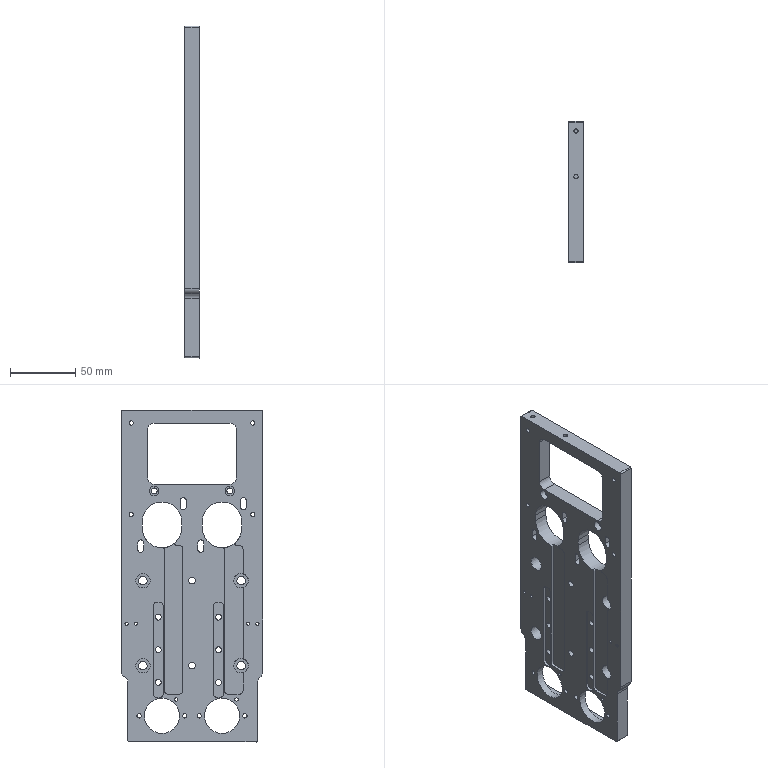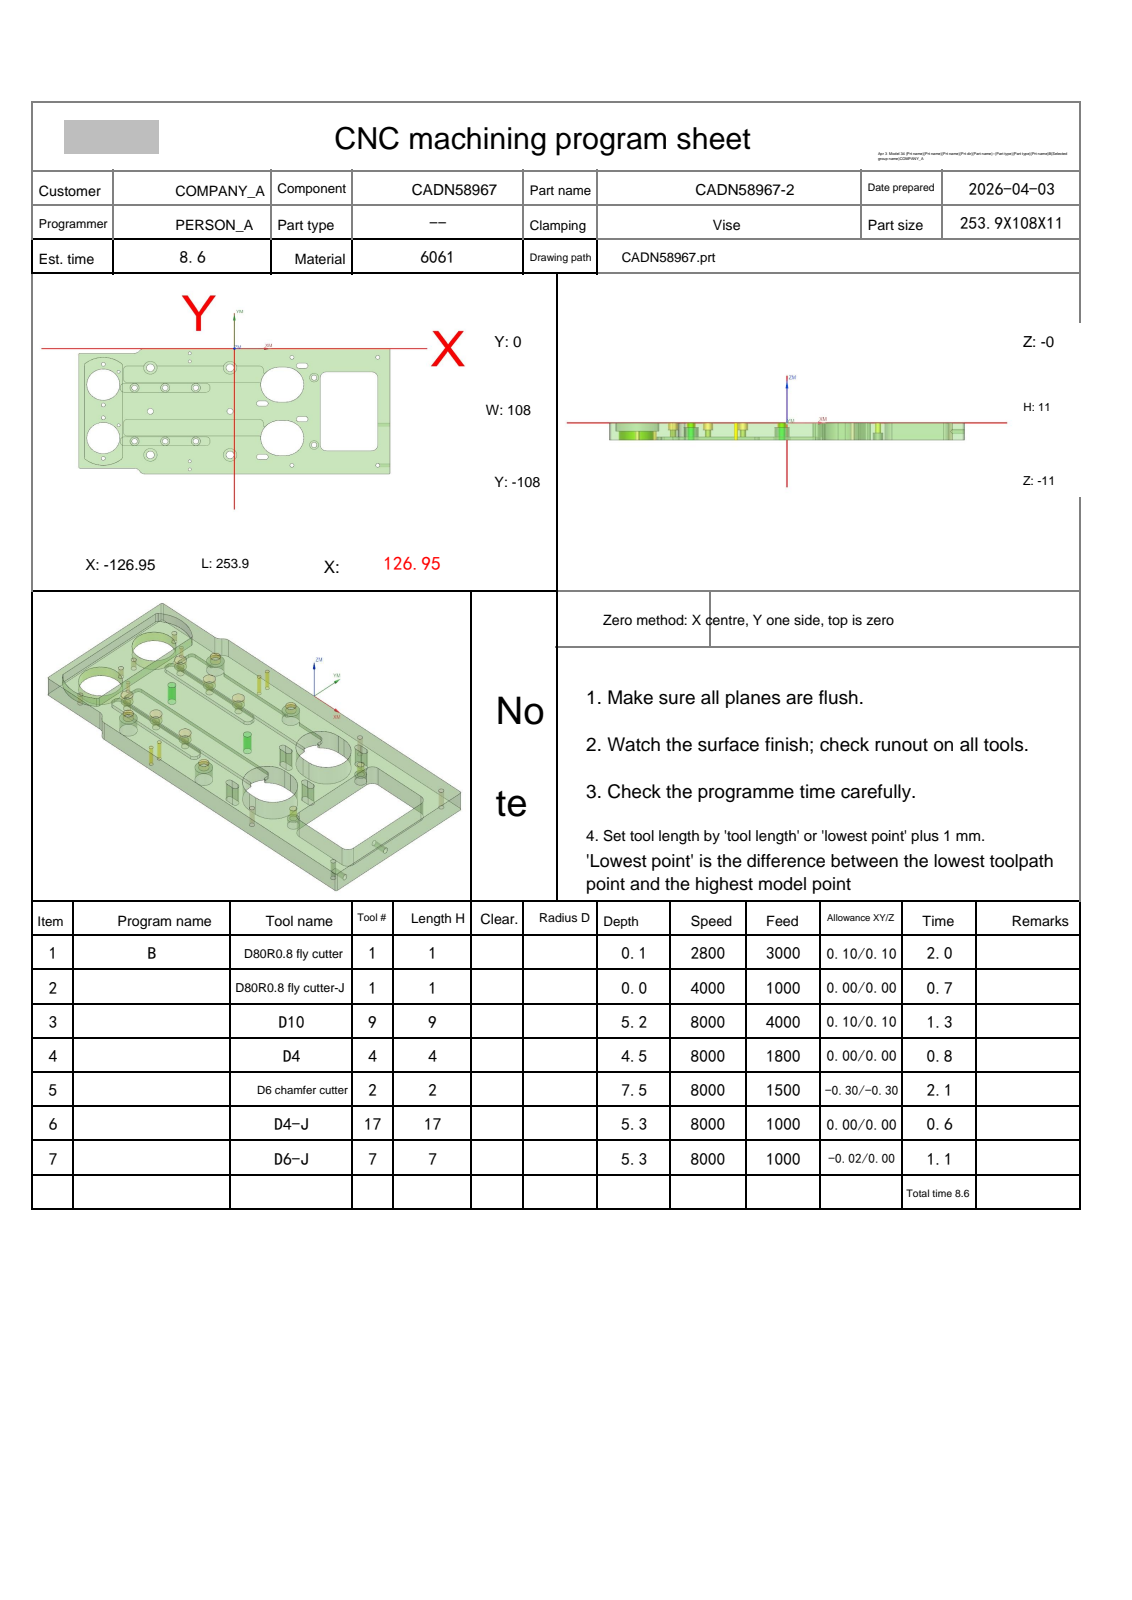NC program | NX | posted by the shop | part box 11 x 108 x 253.9 mm
Lines 1 to 1505 of 3878:
%
O0001
(Machine time: 9.94 MIN)
(===Total Tool:6===)
(T1=D80R0.8 fly cutter D=80.  R=0.8  D-  H01 Z=-0.   )
(T9=D10     D=10.  R=0.   D-  H09 Z=-5.2  )
(T4=D4      D=4.   R=0.   D-  H04 Z=-4.5  )
(T2=D6 chamfer cutter   D=6.   R=0.   D-  H02 Z=-7.5  )
(T17=D4-J   D=4.   R=0.   D-  H17 Z=-5.3  )
(T7=D6-J    D=6.   R=0.   D7  H07 Z=-5.3  )
G80 G90 G17 G49 G40
G91 G28 Z0
M01
N1 T01 M06
(D80R0.8 fly cutter  D=80. R=0.8 H=01 ce=0.10 di=0.10)
G00 G90 G54 X179.047 Y-84.097 M03 S2800
G43 H01 Z20.
M08
Z5.513
G01 Z3.513 F3000.
X167.047
X-159.05
G02 X-167.047 Y-76.101 I.003 J8.
G01 Y-39.263
G02 X-159.047 Y-31.263 I8. J0.0
G01 X167.047
X179.047
Z5.513
G00 Y-84.097
Z5.025
G01 Z3.025
X167.047
X-159.05
G02 X-167.047 Y-76.101 I.003 J8.
G01 Y-39.263
G02 X-159.047 Y-31.263 I8. J0.0
G01 X167.047
X179.047
Z5.025
G00 Y-84.097
Z4.538
G01 Z2.538
X167.047
X-159.05
G02 X-167.047 Y-76.101 I.003 J8.
G01 Y-39.263
G02 X-159.047 Y-31.263 I8. J0.0
G01 X167.047
X179.047
Z4.538
G00 Y-84.097
Z4.05
G01 Z2.05
X167.047
X-159.05
G02 X-167.047 Y-76.101 I.003 J8.
G01 Y-39.263
G02 X-159.047 Y-31.263 I8. J0.0
G01 X167.047
X179.047
Z4.05
G00 Y-84.097
Z3.563
G01 Z1.563
X167.047
X-159.05
G02 X-167.047 Y-76.101 I.003 J8.
G01 Y-39.263
G02 X-159.047 Y-31.263 I8. J0.0
G01 X167.047
X179.047
Z3.563
G00 Y-84.097
Z3.075
G01 Z1.075
X167.047
X-159.05
G02 X-167.047 Y-76.101 I.003 J8.
G01 Y-39.263
G02 X-159.047 Y-31.263 I8. J0.0
G01 X167.047
X179.047
Z3.075
G00 Y-84.097
Z2.588
G01 Z.588
X167.047
X-159.05
G02 X-167.047 Y-76.101 I.003 J8.
G01 Y-39.263
G02 X-159.047 Y-31.263 I8. J0.0
G01 X167.047
X179.047
Z2.588
G00 Y-84.097
Z2.1
G01 Z.1
X167.047
X-159.05
G02 X-167.047 Y-76.101 I.003 J8.
G01 Y-39.263
G02 X-159.047 Y-31.263 I8. J0.0
G01 X167.047
X179.047
Z2.1
G00 Z20.
G91 G28 Z0.0
M05
M09
G91 G28 Z0.0
M01
N2 T01 M06
(D80R0.8 fly cutter-J  D=80. R=0.8 H=01 ce=0.00 di=0.00)
G00 G90 G54 X178.949 Y-83.999 M03 S4000
G43 H01 Z20.
M08
Z2.
G01 Z0.0 F1000.
X166.949
X-158.953
G02 X-166.949 Y-76.003 I.004 J8.
G01 Y-39.361
G02 X-158.949 Y-31.361 I8. J0.0
G01 X166.949
X178.949
Z2.
G00 Z20.
G91 G28 Z0.0
M05
M09
G91 G28 Z0.0
M01
N3 T09 M06
(D10  D=10. R=0. H=09 ce=0.10 di=0.10)
G00 G90 G54 X-104.445 Y-49.592 M03 S8000
G43 H09 Z13.814
M08
Z1.5
G03 X-104.445 Y-49.592 Z.018 I-.905 J-4.408 F4000.
X-109.85 Y-54. Z-.4 I-.905 J-4.408
G01 Y-86.718
G03 X-109.044 Y-87.697 I1. J.002
X-106.95 Y-87.9 I2.094 J10.697
X-104.856 Y-87.697 I0.0 J10.9
X-104.05 Y-86.718 I-.194 J.981
G01 Y-21.282
G03 X-104.856 Y-20.303 I-1. J-.002
X-106.95 Y-20.1 I-2.094 J-10.697
X-109.044 Y-20.303 I0.0 J-10.9
X-109.85 Y-21.282 I.194 J-.981
G01 Y-50.965
G02 X-110.295 Y-51.797 I-1. J0.0
G01 X-116.905 Y-56.203
G03 X-117.35 Y-57.035 I.555 J-.832
G01 Y-92.179
G03 X-106.95 Y-95.4 I10.4 J15.179
X-96.55 Y-92.179 I0.0 J18.4
G01 Y-15.821
G03 X-106.95 Y-12.6 I-10.4 J-15.179
X-117.35 Y-15.821 I0.0 J-18.4
G01 Y-59.
Y-59.5
X-114.35
Z1.1
G00 X-104.445 Y-49.592
G03 X-104.445 Y-49.592 Z-.382 I-.905 J-4.408
X-109.85 Y-54. Z-.8 I-.905 J-4.408
G01 Y-86.718
G03 X-109.044 Y-87.697 I1. J.002
X-106.95 Y-87.9 I2.094 J10.697
X-104.856 Y-87.697 I0.0 J10.9
X-104.05 Y-86.718 I-.194 J.981
G01 Y-21.282
G03 X-104.856 Y-20.303 I-1. J-.002
X-106.95 Y-20.1 I-2.094 J-10.697
X-109.044 Y-20.303 I0.0 J-10.9
X-109.85 Y-21.282 I.194 J-.981
G01 Y-50.965
G02 X-110.295 Y-51.797 I-1. J0.0
G01 X-116.905 Y-56.203
G03 X-117.35 Y-57.035 I.555 J-.832
G01 Y-92.179
G03 X-106.95 Y-95.4 I10.4 J15.179
X-96.55 Y-92.179 I0.0 J18.4
G01 Y-15.821
G03 X-106.95 Y-12.6 I-10.4 J-15.179
X-117.35 Y-15.821 I0.0 J-18.4
G01 Y-59.
Y-59.5
X-114.35
Z.7
G00 X-104.445 Y-49.592
G03 X-104.445 Y-49.592 Z-.782 I-.905 J-4.408
X-109.85 Y-54. Z-1.2 I-.905 J-4.408
G01 Y-86.718
G03 X-109.044 Y-87.697 I1. J.002
X-106.95 Y-87.9 I2.094 J10.697
X-104.856 Y-87.697 I0.0 J10.9
X-104.05 Y-86.718 I-.194 J.981
G01 Y-21.282
G03 X-104.856 Y-20.303 I-1. J-.002
X-106.95 Y-20.1 I-2.094 J-10.697
X-109.044 Y-20.303 I0.0 J-10.9
X-109.85 Y-21.282 I.194 J-.981
G01 Y-50.965
G02 X-110.295 Y-51.797 I-1. J0.0
G01 X-116.905 Y-56.203
G03 X-117.35 Y-57.035 I.555 J-.832
G01 Y-92.179
G03 X-106.95 Y-95.4 I10.4 J15.179
X-96.55 Y-92.179 I0.0 J18.4
G01 Y-15.821
G03 X-106.95 Y-12.6 I-10.4 J-15.179
X-117.35 Y-15.821 I0.0 J-18.4
G01 Y-59.
Y-59.5
X-114.35
Z.3
G00 X-104.445 Y-49.592
G03 X-104.445 Y-49.592 Z-1.182 I-.905 J-4.408
X-109.85 Y-54. Z-1.6 I-.905 J-4.408
G01 Y-86.718
G03 X-109.044 Y-87.697 I1. J.002
X-106.95 Y-87.9 I2.094 J10.697
X-104.856 Y-87.697 I0.0 J10.9
X-104.05 Y-86.718 I-.194 J.981
G01 Y-21.282
G03 X-104.856 Y-20.303 I-1. J-.002
X-106.95 Y-20.1 I-2.094 J-10.697
X-109.044 Y-20.303 I0.0 J-10.9
X-109.85 Y-21.282 I.194 J-.981
G01 Y-50.965
G02 X-110.295 Y-51.797 I-1. J0.0
G01 X-116.905 Y-56.203
G03 X-117.35 Y-57.035 I.555 J-.832
G01 Y-92.179
G03 X-106.95 Y-95.4 I10.4 J15.179
X-96.55 Y-92.179 I0.0 J18.4
G01 Y-15.821
G03 X-106.95 Y-12.6 I-10.4 J-15.179
X-117.35 Y-15.821 I0.0 J-18.4
G01 Y-59.
Y-59.5
X-114.35
Z-.1
G00 X-104.445 Y-49.592
G03 X-104.445 Y-49.592 Z-1.582 I-.905 J-4.408
X-109.85 Y-54. Z-2. I-.905 J-4.408
G01 Y-86.718
G03 X-109.044 Y-87.697 I1. J.002
X-106.95 Y-87.9 I2.094 J10.697
X-104.856 Y-87.697 I0.0 J10.9
X-104.05 Y-86.718 I-.194 J.981
G01 Y-21.282
G03 X-104.856 Y-20.303 I-1. J-.002
X-106.95 Y-20.1 I-2.094 J-10.697
X-109.044 Y-20.303 I0.0 J-10.9
X-109.85 Y-21.282 I.194 J-.981
G01 Y-50.965
G02 X-110.295 Y-51.797 I-1. J0.0
G01 X-116.905 Y-56.203
G03 X-117.35 Y-57.035 I.555 J-.832
G01 Y-92.179
G03 X-106.95 Y-95.4 I10.4 J15.179
X-96.55 Y-92.179 I0.0 J18.4
G01 Y-15.821
G03 X-106.95 Y-12.6 I-10.4 J-15.179
X-117.35 Y-15.821 I0.0 J-18.4
G01 Y-59.
Y-59.5
X-114.35
Z-.5
G00 X-104.445 Y-49.592
G03 X-104.445 Y-49.592 Z-1.982 I-.905 J-4.408
X-109.85 Y-54. Z-2.4 I-.905 J-4.408
G01 Y-86.718
G03 X-109.044 Y-87.697 I1. J.002
X-106.95 Y-87.9 I2.094 J10.697
X-104.856 Y-87.697 I0.0 J10.9
X-104.05 Y-86.718 I-.194 J.981
G01 Y-21.282
G03 X-104.856 Y-20.303 I-1. J-.002
X-106.95 Y-20.1 I-2.094 J-10.697
X-109.044 Y-20.303 I0.0 J-10.9
X-109.85 Y-21.282 I.194 J-.981
G01 Y-50.965
G02 X-110.295 Y-51.797 I-1. J0.0
G01 X-116.905 Y-56.203
G03 X-117.35 Y-57.035 I.555 J-.832
G01 Y-92.179
G03 X-106.95 Y-95.4 I10.4 J15.179
X-96.55 Y-92.179 I0.0 J18.4
G01 Y-15.821
G03 X-106.95 Y-12.6 I-10.4 J-15.179
X-117.35 Y-15.821 I0.0 J-18.4
G01 Y-59.
Y-59.5
X-114.35
Z-.9
G00 X-104.445 Y-49.592
G03 X-104.445 Y-49.592 Z-2.382 I-.905 J-4.408
X-109.85 Y-54. Z-2.8 I-.905 J-4.408
G01 Y-86.718
G03 X-109.044 Y-87.697 I1. J.002
X-106.95 Y-87.9 I2.094 J10.697
X-104.856 Y-87.697 I0.0 J10.9
X-104.05 Y-86.718 I-.194 J.981
G01 Y-21.282
G03 X-104.856 Y-20.303 I-1. J-.002
X-106.95 Y-20.1 I-2.094 J-10.697
X-109.044 Y-20.303 I0.0 J-10.9
X-109.85 Y-21.282 I.194 J-.981
G01 Y-50.965
G02 X-110.295 Y-51.797 I-1. J0.0
G01 X-116.905 Y-56.203
G03 X-117.35 Y-57.035 I.555 J-.832
G01 Y-92.179
G03 X-106.95 Y-95.4 I10.4 J15.179
X-96.55 Y-92.179 I0.0 J18.4
G01 Y-15.821
G03 X-106.95 Y-12.6 I-10.4 J-15.179
X-117.35 Y-15.821 I0.0 J-18.4
G01 Y-59.
Y-59.5
X-114.35
Z-1.3
G00 X-104.445 Y-49.592
G03 X-104.445 Y-49.592 Z-2.782 I-.905 J-4.408
X-109.85 Y-54. Z-3.2 I-.905 J-4.408
G01 Y-86.718
G03 X-109.044 Y-87.697 I1. J.002
X-106.95 Y-87.9 I2.094 J10.697
X-104.856 Y-87.697 I0.0 J10.9
X-104.05 Y-86.718 I-.194 J.981
G01 Y-21.282
G03 X-104.856 Y-20.303 I-1. J-.002
X-106.95 Y-20.1 I-2.094 J-10.697
X-109.044 Y-20.303 I0.0 J-10.9
X-109.85 Y-21.282 I.194 J-.981
G01 Y-50.965
G02 X-110.295 Y-51.797 I-1. J0.0
G01 X-116.905 Y-56.203
G03 X-117.35 Y-57.035 I.555 J-.832
G01 Y-92.179
G03 X-106.95 Y-95.4 I10.4 J15.179
X-96.55 Y-92.179 I0.0 J18.4
G01 Y-15.821
G03 X-106.95 Y-12.6 I-10.4 J-15.179
X-117.35 Y-15.821 I0.0 J-18.4
G01 Y-59.
Y-59.5
X-114.35
Z-1.7
G00 X-104.445 Y-49.592
G03 X-104.445 Y-49.592 Z-3.182 I-.905 J-4.408
X-109.85 Y-54. Z-3.6 I-.905 J-4.408
G01 Y-86.718
G03 X-109.044 Y-87.697 I1. J.002
X-106.95 Y-87.9 I2.094 J10.697
X-104.856 Y-87.697 I0.0 J10.9
X-104.05 Y-86.718 I-.194 J.981
G01 Y-21.282
G03 X-104.856 Y-20.303 I-1. J-.002
X-106.95 Y-20.1 I-2.094 J-10.697
X-109.044 Y-20.303 I0.0 J-10.9
X-109.85 Y-21.282 I.194 J-.981
G01 Y-50.965
G02 X-110.295 Y-51.797 I-1. J0.0
G01 X-116.905 Y-56.203
G03 X-117.35 Y-57.035 I.555 J-.832
G01 Y-92.179
G03 X-106.95 Y-95.4 I10.4 J15.179
X-96.55 Y-92.179 I0.0 J18.4
G01 Y-15.821
G03 X-106.95 Y-12.6 I-10.4 J-15.179
X-117.35 Y-15.821 I0.0 J-18.4
G01 Y-59.
Y-59.5
X-114.35
Z-2.1
G00 X-104.445 Y-49.592
G03 X-104.445 Y-49.592 Z-3.582 I-.905 J-4.408
X-109.85 Y-54. Z-4. I-.905 J-4.408
G01 Y-86.718
G03 X-109.044 Y-87.697 I1. J.002
X-106.95 Y-87.9 I2.094 J10.697
X-104.856 Y-87.697 I0.0 J10.9
X-104.05 Y-86.718 I-.194 J.981
G01 Y-21.282
G03 X-104.856 Y-20.303 I-1. J-.002
X-106.95 Y-20.1 I-2.094 J-10.697
X-109.044 Y-20.303 I0.0 J-10.9
X-109.85 Y-21.282 I.194 J-.981
G01 Y-50.965
G02 X-110.295 Y-51.797 I-1. J0.0
G01 X-116.905 Y-56.203
G03 X-117.35 Y-57.035 I.555 J-.832
G01 Y-92.179
G03 X-106.95 Y-95.4 I10.4 J15.179
X-96.55 Y-92.179 I0.0 J18.4
G01 Y-15.821
G03 X-106.95 Y-12.6 I-10.4 J-15.179
X-117.35 Y-15.821 I0.0 J-18.4
G01 Y-59.
Y-59.5
X-114.35
Z-2.5
G00 X-104.445 Y-49.592
G03 X-104.445 Y-49.592 Z-3.982 I-.905 J-4.408
X-109.85 Y-54. Z-4.4 I-.905 J-4.408
G01 Y-86.718
G03 X-109.044 Y-87.697 I1. J.002
X-106.95 Y-87.9 I2.094 J10.697
X-104.856 Y-87.697 I0.0 J10.9
X-104.05 Y-86.718 I-.194 J.981
G01 Y-21.282
G03 X-104.856 Y-20.303 I-1. J-.002
X-106.95 Y-20.1 I-2.094 J-10.697
X-109.044 Y-20.303 I0.0 J-10.9
X-109.85 Y-21.282 I.194 J-.981
G01 Y-50.965
G02 X-110.295 Y-51.797 I-1. J0.0
G01 X-116.905 Y-56.203
G03 X-117.35 Y-57.035 I.555 J-.832
G01 Y-92.179
G03 X-106.95 Y-95.4 I10.4 J15.179
X-96.55 Y-92.179 I0.0 J18.4
G01 Y-15.821
G03 X-106.95 Y-12.6 I-10.4 J-15.179
X-117.35 Y-15.821 I0.0 J-18.4
G01 Y-59.
Y-59.5
X-114.35
Z-2.9
G00 X-104.445 Y-49.592
G03 X-104.445 Y-49.592 Z-4.382 I-.905 J-4.408
X-109.85 Y-54. Z-4.8 I-.905 J-4.408
G01 Y-86.718
G03 X-109.044 Y-87.697 I1. J.002
X-106.95 Y-87.9 I2.094 J10.697
X-104.856 Y-87.697 I0.0 J10.9
X-104.05 Y-86.718 I-.194 J.981
G01 Y-21.282
G03 X-104.856 Y-20.303 I-1. J-.002
X-106.95 Y-20.1 I-2.094 J-10.697
X-109.044 Y-20.303 I0.0 J-10.9
X-109.85 Y-21.282 I.194 J-.981
G01 Y-50.965
G02 X-110.295 Y-51.797 I-1. J0.0
G01 X-116.905 Y-56.203
G03 X-117.35 Y-57.035 I.555 J-.832
G01 Y-92.179
G03 X-106.95 Y-95.4 I10.4 J15.179
X-96.55 Y-92.179 I0.0 J18.4
G01 Y-15.821
G03 X-106.95 Y-12.6 I-10.4 J-15.179
X-117.35 Y-15.821 I0.0 J-18.4
G01 Y-59.
Y-59.5
X-114.35
Z-3.3
G00 X-104.445 Y-49.592
G03 X-104.445 Y-49.592 Z-4.782 I-.905 J-4.408
X-109.85 Y-54. Z-5.2 I-.905 J-4.408
G01 Y-86.718
G03 X-109.044 Y-87.697 I1. J.002
X-106.95 Y-87.9 I2.094 J10.697
X-104.856 Y-87.697 I0.0 J10.9
X-104.05 Y-86.718 I-.194 J.981
G01 Y-21.282
G03 X-104.856 Y-20.303 I-1. J-.002
X-106.95 Y-20.1 I-2.094 J-10.697
X-109.044 Y-20.303 I0.0 J-10.9
X-109.85 Y-21.282 I.194 J-.981
G01 Y-50.965
G02 X-110.295 Y-51.797 I-1. J0.0
G01 X-116.905 Y-56.203
G03 X-117.35 Y-57.035 I.555 J-.832
G01 Y-92.179
G03 X-106.95 Y-95.4 I10.4 J15.179
X-96.55 Y-92.179 I0.0 J18.4
G01 Y-15.821
G03 X-106.95 Y-12.6 I-10.4 J-15.179
X-117.35 Y-15.821 I0.0 J-18.4
G01 Y-59.
Y-59.5
X-114.35
Z-3.7
G00 Z13.814
G91 G28 Z0.0
M05
M09
G91 G28 Z0.0
M01
N4 T04 M06
(D4  D=4. R=0. H=04 ce=0.07 di=0.00)
G00 G90 G54 X-56.45 Y-79.75 M03 S8000
G43 H04 Z20.
M08
Z.3
G03 X-57.29 Y-80.59 I0.0 J-.84 F1800.
X-56.45 Y-81.43 I.84 J0.0
X-56.45 Y-81.43 Z-.05 I0.0 J1.68
X-56.45 Y-81.43 Z-.4 I0.0 J1.68
X-56.45 Y-81.43 Z-.75 I0.0 J1.68
X-56.45 Y-81.43 Z-1.1 I0.0 J1.68
X-56.45 Y-81.43 Z-1.45 I0.0 J1.68
X-56.45 Y-81.43 Z-1.8 I0.0 J1.68
X-56.45 Y-81.43 Z-2.15 I0.0 J1.68
X-56.45 Y-81.43 Z-2.5 I0.0 J1.68
X-56.45 Y-81.43 Z-2.85 I0.0 J1.68
X-56.45 Y-81.43 Z-3.2 I0.0 J1.68
X-56.45 Y-81.43 Z-3.55 I0.0 J1.68
X-56.45 Y-81.43 Z-3.9 I0.0 J1.68
X-56.45 Y-81.43 Z-4.25 I0.0 J1.68
X-58.088 Y-79.376 Z-4.5 I0.0 J1.68
X-58.13 Y-79.75 I1.638 J-.374
X-56.45 Y-81.43 I1.68 J0.0
X-54.77 Y-79.75 I0.0 J1.68
X-56.45 Y-78.07 I-1.68 J0.0
X-58.088 Y-79.376 I0.0 J-1.68
G01 X-58.109 Y-79.563
G03 X-57.269 Y-80.403 I.84 J0.0
X-56.45 Y-79.75 I0.0 J.84
G00 Z20.
X-31.45
Z.3
G03 X-32.29 Y-80.59 I0.0 J-.84
X-31.45 Y-81.43 I.84 J0.0
X-31.45 Y-81.43 Z-.05 I0.0 J1.68
X-31.45 Y-81.43 Z-.4 I0.0 J1.68
X-31.45 Y-81.43 Z-.75 I0.0 J1.68
X-31.45 Y-81.43 Z-1.1 I0.0 J1.68
X-31.45 Y-81.43 Z-1.45 I0.0 J1.68
X-31.45 Y-81.43 Z-1.8 I0.0 J1.68
X-31.45 Y-81.43 Z-2.15 I0.0 J1.68
X-31.45 Y-81.43 Z-2.5 I0.0 J1.68
X-31.45 Y-81.43 Z-2.85 I0.0 J1.68
X-31.45 Y-81.43 Z-3.2 I0.0 J1.68
X-31.45 Y-81.43 Z-3.55 I0.0 J1.68
X-31.45 Y-81.43 Z-3.9 I0.0 J1.68
X-31.45 Y-81.43 Z-4.25 I0.0 J1.68
X-33.088 Y-79.376 Z-4.5 I0.0 J1.68
X-33.13 Y-79.75 I1.638 J-.374
X-31.45 Y-81.43 I1.68 J0.0
X-29.77 Y-79.75 I0.0 J1.68
X-31.45 Y-78.07 I-1.68 J0.0
X-33.088 Y-79.376 I0.0 J-1.68
G01 X-33.109 Y-79.563
G03 X-32.269 Y-80.403 I.84 J0.0
X-31.45 Y-79.75 I0.0 J.84
G00 Z20.
Y-33.75
Z.3
G03 X-32.29 Y-34.59 I0.0 J-.84
X-31.45 Y-35.43 I.84 J0.0
X-31.45 Y-35.43 Z-.05 I0.0 J1.68
X-31.45 Y-35.43 Z-.4 I0.0 J1.68
X-31.45 Y-35.43 Z-.75 I0.0 J1.68
X-31.45 Y-35.43 Z-1.1 I0.0 J1.68
X-31.45 Y-35.43 Z-1.45 I0.0 J1.68
X-31.45 Y-35.43 Z-1.8 I0.0 J1.68
X-31.45 Y-35.43 Z-2.15 I0.0 J1.68
X-31.45 Y-35.43 Z-2.5 I0.0 J1.68
X-31.45 Y-35.43 Z-2.85 I0.0 J1.68
X-31.45 Y-35.43 Z-3.2 I0.0 J1.68
X-31.45 Y-35.43 Z-3.55 I0.0 J1.68
X-31.45 Y-35.43 Z-3.9 I0.0 J1.68
X-31.45 Y-35.43 Z-4.25 I0.0 J1.68
X-33.088 Y-33.376 Z-4.5 I0.0 J1.68
X-33.13 Y-33.75 I1.638 J-.374
X-31.45 Y-35.43 I1.68 J0.0
X-29.77 Y-33.75 I0.0 J1.68
X-31.45 Y-32.07 I-1.68 J0.0
X-33.088 Y-33.376 I0.0 J-1.68
G01 X-33.109 Y-33.563
G03 X-32.269 Y-34.403 I.84 J0.0
X-31.45 Y-33.75 I0.0 J.84
G00 Z20.
X-56.45
Z.3
G03 X-57.29 Y-34.59 I0.0 J-.84
X-56.45 Y-35.43 I.84 J0.0
X-56.45 Y-35.43 Z-.05 I0.0 J1.68
X-56.45 Y-35.43 Z-.4 I0.0 J1.68
X-56.45 Y-35.43 Z-.75 I0.0 J1.68
X-56.45 Y-35.43 Z-1.1 I0.0 J1.68
X-56.45 Y-35.43 Z-1.45 I0.0 J1.68
X-56.45 Y-35.43 Z-1.8 I0.0 J1.68
X-56.45 Y-35.43 Z-2.15 I0.0 J1.68
X-56.45 Y-35.43 Z-2.5 I0.0 J1.68
X-56.45 Y-35.43 Z-2.85 I0.0 J1.68
X-56.45 Y-35.43 Z-3.2 I0.0 J1.68
X-56.45 Y-35.43 Z-3.55 I0.0 J1.68
X-56.45 Y-35.43 Z-3.9 I0.0 J1.68
X-56.45 Y-35.43 Z-4.25 I0.0 J1.68
X-58.088 Y-33.376 Z-4.5 I0.0 J1.68
X-58.13 Y-33.75 I1.638 J-.374
X-56.45 Y-35.43 I1.68 J0.0
X-54.77 Y-33.75 I0.0 J1.68
X-56.45 Y-32.07 I-1.68 J0.0
X-58.088 Y-33.376 I0.0 J-1.68
G01 X-58.109 Y-33.563
G03 X-57.269 Y-34.403 I.84 J0.0
X-56.45 Y-33.75 I0.0 J.84
G00 Z20.
X-81.45
Z.3
G03 X-82.29 Y-34.59 I0.0 J-.84
X-81.45 Y-35.43 I.84 J0.0
X-81.45 Y-35.43 Z-.05 I0.0 J1.68
X-81.45 Y-35.43 Z-.4 I0.0 J1.68
X-81.45 Y-35.43 Z-.75 I0.0 J1.68
X-81.45 Y-35.43 Z-1.1 I0.0 J1.68
X-81.45 Y-35.43 Z-1.45 I0.0 J1.68
X-81.45 Y-35.43 Z-1.8 I0.0 J1.68
X-81.45 Y-35.43 Z-2.15 I0.0 J1.68
X-81.45 Y-35.43 Z-2.5 I0.0 J1.68
X-81.45 Y-35.43 Z-2.85 I0.0 J1.68
X-81.45 Y-35.43 Z-3.2 I0.0 J1.68
X-81.45 Y-35.43 Z-3.55 I0.0 J1.68
X-81.45 Y-35.43 Z-3.9 I0.0 J1.68
X-81.45 Y-35.43 Z-4.25 I0.0 J1.68
X-83.088 Y-33.376 Z-4.5 I0.0 J1.68
X-83.13 Y-33.75 I1.638 J-.374
X-81.45 Y-35.43 I1.68 J0.0
X-79.77 Y-33.75 I0.0 J1.68
X-81.45 Y-32.07 I-1.68 J0.0
X-83.088 Y-33.376 I0.0 J-1.68
G01 X-83.109 Y-33.563
G03 X-82.269 Y-34.403 I.84 J0.0
X-81.45 Y-33.75 I0.0 J.84
G00 Z20.
Y-79.75
Z.3
G03 X-82.29 Y-80.59 I0.0 J-.84
X-81.45 Y-81.43 I.84 J0.0
X-81.45 Y-81.43 Z-.05 I0.0 J1.68
X-81.45 Y-81.43 Z-.4 I0.0 J1.68
X-81.45 Y-81.43 Z-.75 I0.0 J1.68
X-81.45 Y-81.43 Z-1.1 I0.0 J1.68
X-81.45 Y-81.43 Z-1.45 I0.0 J1.68
X-81.45 Y-81.43 Z-1.8 I0.0 J1.68
X-81.45 Y-81.43 Z-2.15 I0.0 J1.68
X-81.45 Y-81.43 Z-2.5 I0.0 J1.68
X-81.45 Y-81.43 Z-2.85 I0.0 J1.68
X-81.45 Y-81.43 Z-3.2 I0.0 J1.68
X-81.45 Y-81.43 Z-3.55 I0.0 J1.68
X-81.45 Y-81.43 Z-3.9 I0.0 J1.68
X-81.45 Y-81.43 Z-4.25 I0.0 J1.68
X-83.088 Y-79.376 Z-4.5 I0.0 J1.68
X-83.13 Y-79.75 I1.638 J-.374
X-81.45 Y-81.43 I1.68 J0.0
X-79.77 Y-79.75 I0.0 J1.68
X-81.45 Y-78.07 I-1.68 J0.0
X-83.088 Y-79.376 I0.0 J-1.68
G01 X-83.109 Y-79.563
G03 X-82.269 Y-80.403 I.84 J0.0
X-81.45 Y-79.75 I0.0 J.84
G00 Z20.
G00 G90 X-56.45 Y-79.75 M03 S8000
Z20.
Z-4.5
G01 X-56.772 Y-81.092 F600.
X-56.781 Y-81.169
G03 X-56.45 Y-81.5 I.331 J0.0
X-54.7 Y-79.75 I0.0 J1.75
X-56.45 Y-78. I-1.75 J0.0
X-58.2 Y-79.75 I0.0 J-1.75
X-56.45 Y-81.5 I1.75 J0.0
X-55.957 Y-81.429 I0.0 J1.75
X-55.719 Y-81.112 I-.093 J.317
G01 X-55.763 Y-80.947
X-56.45 Y-79.75
G00 Z20.
X-31.45
Z-4.5
G01 X-31.772 Y-81.092
X-31.781 Y-81.169
G03 X-31.45 Y-81.5 I.331 J0.0
X-29.7 Y-79.75 I0.0 J1.75
X-31.45 Y-78. I-1.75 J0.0
X-33.2 Y-79.75 I0.0 J-1.75
X-31.45 Y-81.5 I1.75 J0.0
X-30.957 Y-81.429 I0.0 J1.75
X-30.719 Y-81.112 I-.093 J.317
G01 X-30.763 Y-80.947
X-31.45 Y-79.75
G00 Z20.
Y-33.75
Z-4.5
G01 X-31.772 Y-35.092
X-31.781 Y-35.169
G03 X-31.45 Y-35.5 I.331 J0.0
X-29.7 Y-33.75 I0.0 J1.75
X-31.45 Y-32. I-1.75 J0.0
X-33.2 Y-33.75 I0.0 J-1.75
X-31.45 Y-35.5 I1.75 J0.0
X-30.957 Y-35.429 I0.0 J1.75
X-30.719 Y-35.112 I-.093 J.317
G01 X-30.763 Y-34.947
X-31.45 Y-33.75
G00 Z20.
X-56.45
Z-4.5
G01 X-56.772 Y-35.092
X-56.781 Y-35.169
G03 X-56.45 Y-35.5 I.331 J0.0
X-54.7 Y-33.75 I0.0 J1.75
X-56.45 Y-32. I-1.75 J0.0
X-58.2 Y-33.75 I0.0 J-1.75
X-56.45 Y-35.5 I1.75 J0.0
X-55.957 Y-35.429 I0.0 J1.75
X-55.719 Y-35.112 I-.093 J.317
G01 X-55.763 Y-34.947
X-56.45 Y-33.75
G00 Z20.
X-81.45
Z-4.5
G01 X-81.772 Y-35.092
X-81.781 Y-35.169
G03 X-81.45 Y-35.5 I.331 J0.0
X-79.7 Y-33.75 I0.0 J1.75
X-81.45 Y-32. I-1.75 J0.0
X-83.2 Y-33.75 I0.0 J-1.75
X-81.45 Y-35.5 I1.75 J0.0
X-80.957 Y-35.429 I0.0 J1.75
X-80.719 Y-35.112 I-.093 J.317
G01 X-80.763 Y-34.947
X-81.45 Y-33.75
G00 Z20.
Y-79.75
Z-4.5
G01 X-81.772 Y-81.092
X-81.781 Y-81.169
G03 X-81.45 Y-81.5 I.331 J0.0
X-79.7 Y-79.75 I0.0 J1.75
X-81.45 Y-78. I-1.75 J0.0
X-83.2 Y-79.75 I0.0 J-1.75
X-81.45 Y-81.5 I1.75 J0.0
X-80.957 Y-81.429 I0.0 J1.75
X-80.719 Y-81.112 I-.093 J.317
G01 X-80.763 Y-80.947
X-81.45 Y-79.75
G00 Z20.
G91 G28 Z0.0
M05
M09
G91 G28 Z0.0
M01
N5 T02 M06
(D6 chamfer cutter  D=6. R=0. H=02 ce=-0.30 di=0.00)
G00 G90 G54 X84.666 Y-20.7 M03 S7000
G43 H02 Z20.
M08
Z2.5
G01 X75.05 Z-1. F1500.
G03 X70.75 Y-25. I0.0 J-4.3
G01 Y-83.
G03 X75.05 Y-87.3 I4.3 J0.0
G01 X111.95
G03 X116.25 Y-83. I0.0 J4.3
G01 Y-25.
G03 X111.95 Y-20.7 I-4.3 J0.0
G01 X75.05
G03 X74.551 Y-20.729 I0.0 J-4.3
G01 Z1.5
G00 Z20.
X46.087 Y-63.335
Z2.5
G01 X45.858 Y-63.256 Z2.412
X45.073 Y-63.034 Z2.115
X44.276 Y-62.857 Z1.818
X43.471 Y-62.726 Z1.521
X42.659 Y-62.64 Z1.224
X41.844 Y-62.6 Z.927
X36.55 Z-1.
G03 X22.15 Y-77. I0.0 J-14.4
X36.55 Y-91.4 I14.4 J0.0
G01 X41.55
G03 X55.95 Y-77. I0.0 J14.4
X41.55 Y-62.6 I-14.4 J0.0
G01 X36.55
G03 X36.05 Y-62.609 I0.0 J-14.4
G01 Z1.5
G00 Z20.
X46.087 Y-17.335
Z2.5
G01 X45.858 Y-17.256 Z2.412
X45.073 Y-17.034 Z2.115
X44.276 Y-16.857 Z1.818
X43.471 Y-16.726 Z1.521
X42.659 Y-16.64 Z1.224
X41.844 Y-16.6 Z.927
X36.55 Z-1.
G03 X22.15 Y-31. I0.0 J-14.4
X36.55 Y-45.4 I14.4 J0.0
G01 X41.55
G03 X55.95 Y-31. I0.0 J14.4
X41.55 Y-16.6 I-14.4 J0.0
G01 X36.55
G03 X36.05 Y-16.609 I0.0 J-14.4
G01 Z1.5
G00 Z20.
G00 G90 X-36.45 Y-104. M03 S8000
Z20.
G98 G81 X-36.45 Y-104. Z-1.75 R3. F1000.
Y-97.
X-94.45 Y-65.955 Z-7.05 R-2.3
Y-19.955
X-36.45 Y-11. Z-1.75 R3.
Y-4.
G80
G00 Z20.
G00 G90 X116.95 Y-7.5 M03 S8000
Z20.
G98 G81 X116.95 Y-7.5 Z-2.2 R3. F1000.
X46.95
Y-100.5
X-106.95 Y-94.5 Z-7.5 R-2.3
Y-59.5
Y-48.5
Y-13.5
G80
G00 Z20.
G00 G90 X65.05 Y-25. M03 S8000
Z20.
G98 G81 X65.05 Y-25. Z-2.55 R3. F1000.
Y-83.
G80
G00 Z20.
G00 G90 X-68.389 Y-54.377 M03 S8000
Z20.
Z-.9
G01 Z-1.4 F1200.
X-68.221 Y-54.386
X-68.146 Y-54.388
G03 X-67.14 Y-54. I0.0 J1.5
X-68.55 Y-52.59 I-1.41 J0.0
X-69.96 Y-54. I0.0 J-1.41
X-68.55 Y-55.41 I1.41 J0.0
X-67.14 Y-54. I0.0 J1.41
X-68.146 Y-53.612 I-1.006 J-1.112
G01 X-68.221 Y-53.614
X-68.389 Y-53.623
Z-.9
G00 Z20.
X-3.389 Y-54.377
Z-.9
G01 Z-1.4
X-3.221 Y-54.386
X-3.146 Y-54.388
G03 X-2.14 Y-54. I0.0 J1.5
X-3.55 Y-52.59 I-1.41 J0.0
X-4.96 Y-54. I0.0 J-1.41
X-3.55 Y-55.41 I1.41 J0.0
X-2.14 Y-54. I0.0 J1.41
X-3.146 Y-53.612 I-1.006 J-1.112
G01 X-3.221 Y-53.614
X-3.389 Y-53.623
Z-.9
G00 Z20.
G00 G90 X-69.007 Y-90.445 M03 S8000
Z20.
Z-.9
G01 Z-1.4 F1200.
X-69.2 Y-90.
G03 X-70.7 Y-91.5 I0.0 J-1.5
X-68.55 Y-93.65 I2.15 J0.0
X-66.4 Y-91.5 I0.0 J2.15
X-68.55 Y-89.35 I-2.15 J0.0
X-70.7 Y-91.5 I0.0 J-2.15
X-69.2 Y-93. I1.5 J0.0
G01 X-69.007 Y-92.555
Z-.9
G00 Z20.
X-4.007 Y-90.445
Z-.9
G01 Z-1.4
X-4.2 Y-90.
G03 X-5.7 Y-91.5 I0.0 J-1.5
X-3.55 Y-93.65 I2.15 J0.0
X-1.4 Y-91.5 I0.0 J2.15
X-3.55 Y-89.35 I-2.15 J0.0
X-5.7 Y-91.5 I0.0 J-2.15
X-4.2 Y-93. I1.5 J0.0
G01 X-4.007 Y-92.555
Z-.9
G00 Z20.
Y-15.445
Z-.9
G01 Z-1.4
X-4.2 Y-15.
G03 X-5.7 Y-16.5 I0.0 J-1.5
X-3.55 Y-18.65 I2.15 J0.0
X-1.4 Y-16.5 I0.0 J2.15
X-3.55 Y-14.35 I-2.15 J0.0
X-5.7 Y-16.5 I0.0 J-2.15
X-4.2 Y-18. I1.5 J0.0
G01 X-4.007 Y-17.555
Z-.9
G00 Z20.
X-69.007 Y-15.445
Z-.9
G01 Z-1.4
X-69.2 Y-15.
G03 X-70.7 Y-16.5 I0.0 J-1.5
X-68.55 Y-18.65 I2.15 J0.0
X-66.4 Y-16.5 I0.0 J2.15
X-68.55 Y-14.35 I-2.15 J0.0
X-70.7 Y-16.5 I0.0 J-2.15
X-69.2 Y-18. I1.5 J0.0
G01 X-69.007 Y-17.555
Z-.9
G00 Z20.
G00 G90 X25.814 Y1.227 M03 S6500
Z20.
Z.172
G01 Z-1.199 F1500.
G03 X26.1 Y1.027 I1.286 J1.532
G01 X26.146 Y.997
X26.2 Y1.
X125.95
G02 X127.95 Y-1. I0.0 J-2.
G01 Y-107.001
G02 X125.95 Y-109. I-2. J.001
G01 X-72.89
G02 X-78.086 Y-106. I0.0 J6.
G03 X-81.55 Y-104. I-3.464 J-2.
G01 X-125.95
G02 X-127.95 Y-102. I0.0 J2.
G01 Y-5.
G02 X-125.95 Y-3. I2. J0.0
G01 X-81.55
G03 X-78.35 Y-1.4 I0.0 J4.
G02 X-73.55 Y1. I4.8 J-3.6
G01 X26.2
X26.254 Y.997
X26.3 Y1.027
G03 X26.586 Y1.227 I-1. J1.732
G01 Z.172
G00 Z10.
X117.444 Y-7.919
Z.405
G01 Z-1.199
G03 X117.591 Y-7.603 I-1.732 J1.
G01 X117.612 Y-7.553
X117.6 Y-7.5
G03 X116.95 Y-6.85 I-.65 J0.0
X116.3 Y-7.5 I0.0 J-.65
X116.95 Y-8.15 I.65 J0.0
X117.6 Y-7.5 I0.0 J.65
G01 X117.612 Y-7.447
X117.591 Y-7.397
G03 X117.444 Y-7.081 I-1.879 J-.684
G01 Z.405
G00 Z10.
X63.985 Y-24.593
Z.294
G01 Z-1.199
G03 X63.816 Y-24.898 I1.658 J-1.118
G01 X63.791 Y-24.946
X63.8 Y-25.
G03 X65.05 Y-26.25 I1.25 J0.0
X66.3 Y-25. I0.0 J1.25
X65.05 Y-23.75 I-1.25 J0.0
X63.827 Y-24.74 I0.0 J-1.25
G01 X63.8 Y-25.
X63.791 Y-25.054
X63.816 Y-25.102
G03 X63.985 Y-25.407 I1.827 J.813
G01 Z.294
G00 Z10.
X54.901 Y-15.76
Z.172
G01 Z-1.199
G03 X55.187 Y-15.96 I1.286 J1.532
G01 X55.232 Y-15.989
X55.287 Y-15.987
X57.787
G03 X59.037 Y-14.737 I0.0 J1.25
X57.787 Y-13.487 I-1.25 J0.0
G01 X52.787
G03 X51.537 Y-14.737 I0.0 J-1.25
X52.787 Y-15.987 I1.25 J0.0
G01 X55.287
X55.341 Y-15.989
X55.387 Y-15.96
G03 X55.672 Y-15.76 I-1. J1.732
G01 Z.172
G00 Z2.551
X47.444 Y-7.919
Z.405
G01 Z-1.199
G03 X47.591 Y-7.603 I-1.732 J1.
G01 X47.612 Y-7.553
X47.6 Y-7.5
G03 X46.95 Y-6.85 I-.65 J0.0
X46.3 Y-7.5 I0.0 J-.65
X46.95 Y-8.15 I.65 J0.0
X47.6 Y-7.5 I0.0 J.65
G01 X47.612 Y-7.447
X47.591 Y-7.397
G03 X47.444 Y-7.081 I-1.879 J-.684
G01 Z.405
G00 Z10.
X39.436 Y-17.127
Z.172
G01 Z-1.199
G03 X39.15 Y-16.927 I-1.286 J-1.532
G01 X39.104 Y-16.897
X39.05 Y-16.9
X36.55
G03 X22.45 Y-31. I0.0 J-14.1
X36.55 Y-45.1 I14.1 J0.0
G01 X41.55
G03 X55.65 Y-31. I0.0 J14.1
X41.55 Y-16.9 I-14.1 J0.0
G01 X39.05
X38.996 Y-16.897
X38.95 Y-16.927
G03 X38.664 Y-17.127 I1. J-1.732
G01 Z.172
G00 Z10.
X23.199 Y-46.24
Z.172
G01 Z-1.199
G03 X22.913 Y-46.04 I-1.286 J-1.532
G01 X22.868 Y-46.011
X22.813 Y-46.013
X20.313
G03 X19.063 Y-47.263 I0.0 J-1.25
X20.313 Y-48.513 I1.25 J0.0
G01 X25.313
G03 X26.563 Y-47.263 I0.0 J1.25
X25.313 Y-46.013 I-1.25 J0.0
G01 X22.813
X22.759 Y-46.011
X22.713 Y-46.04
G03 X22.428 Y-46.24 I1. J-1.732
G01 Z.172
G00 Z10.
X-2.225 Y-54.407
Z.283
G01 Z-1.199
G03 X-2.056 Y-54.102 I-1.658 J1.118
G01 X-2.031 Y-54.054
X-2.04 Y-54.
G03 X-3.55 Y-52.49 I-1.51 J0.0
X-5.06 Y-54. I0.0 J-1.51
X-3.55 Y-55.51 I1.51 J0.0
X-2.04 Y-54. I0.0 J1.51
G01 X-2.031 Y-53.946
X-2.056 Y-53.898
G03 X-2.225 Y-53.593 I-1.827 J-.813
G01 Z.283
G00 Z10.
X-5.608 Y-16.096
Z.253
G01 Z-1.199
G03 X-5.782 Y-16.398 I1.638 J-1.147
G01 X-5.808 Y-16.446
X-5.8 Y-16.5
G03 X-3.55 Y-18.75 I2.25 J0.0
X-1.3 Y-16.5 I0.0 J2.25
X-3.55 Y-14.25 I-2.25 J0.0
X-5.8 Y-16.5 I0.0 J-2.25
G01 X-5.808 Y-16.554
X-5.782 Y-16.602
G03 X-5.608 Y-16.904 I1.813 J.845
G01 Z.253
G00 Z10.
X-28.897 Y-34.151
Z.238
G01 Z-1.199
G03 X-28.719 Y-33.852 I-1.624 J1.167
G01 X-28.693 Y-33.804
X-28.7 Y-33.75
G03 X-31.45 Y-31. I-2.75 J0.0
X-34.2 Y-33.75 I0.0 J-2.75
X-31.45 Y-36.5 I2.75 J0.0
X-28.7 Y-33.75 I0.0 J2.75
G01 X-28.693 Y-33.696
X-28.719 Y-33.648
G03 X-28.897 Y-33.349 I-1.802 J-.868
G01 Z.238
G00 Z10.
X-53.897 Y-34.151
Z.238
G01 Z-1.199
G03 X-53.719 Y-33.852 I-1.624 J1.167
G01 X-53.693 Y-33.804
X-53.7 Y-33.75
G03 X-56.45 Y-31. I-2.75 J0.0
X-59.2 Y-33.75 I0.0 J-2.75
X-56.45 Y-36.5 I2.75 J0.0
X-53.7 Y-33.75 I0.0 J2.75
G01 X-53.693 Y-33.696
X-53.719 Y-33.648
G03 X-53.897 Y-33.349 I-1.802 J-.868
G01 Z.238
G00 Z10.
X-70.608 Y-16.096
Z.253
G01 Z-1.199
G03 X-70.782 Y-16.398 I1.638 J-1.147
G01 X-70.808 Y-16.446
X-70.8 Y-16.5
G03 X-68.55 Y-18.75 I2.25 J0.0
X-66.3 Y-16.5 I0.0 J2.25
X-68.55 Y-14.25 I-2.25 J0.0
X-70.8 Y-16.5 I0.0 J-2.25
G01 X-70.808 Y-16.554
X-70.782 Y-16.602
G03 X-70.608 Y-16.904 I1.813 J.845
G01 Z.253
G00 Z10.
X-78.897 Y-34.151
Z.238
G01 Z-1.199
G03 X-78.719 Y-33.852 I-1.624 J1.167
G01 X-78.693 Y-33.804
X-78.7 Y-33.75
G03 X-81.45 Y-31. I-2.75 J0.0
X-84.2 Y-33.75 I0.0 J-2.75
X-81.45 Y-36.5 I2.75 J0.0
X-78.7 Y-33.75 I0.0 J2.75
G01 X-78.693 Y-33.696
X-78.719 Y-33.648
G03 X-78.897 Y-33.349 I-1.802 J-.868
G01 Z.238
G00 Z10.
X-67.225 Y-54.407
Z.283
G01 Z-1.199
G03 X-67.056 Y-54.102 I-1.658 J1.118
G01 X-67.031 Y-54.054
X-67.04 Y-54.
G03 X-68.55 Y-52.49 I-1.51 J0.0
X-70.06 Y-54. I0.0 J-1.51
X-68.55 Y-55.51 I1.51 J0.0
X-67.04 Y-54. I0.0 J1.51
G01 X-67.031 Y-53.946
X-67.056 Y-53.898
G03 X-67.225 Y-53.593 I-1.827 J-.813
G01 Z.283
G00 Z10.
X-121.223 Y-53.614
Z.172
G01 Z-1.199
G03 X-121.423 Y-53.9 I1.532 J-1.286
G01 X-121.453 Y-53.946
X-121.45 Y-54.
Y-93.733
X-121.425 Y-93.954
X-121.352 Y-94.165
X-121.234 Y-94.353
X-121.078 Y-94.511
G03 X-106.95 Y-99.5 I14.128 J17.511
X-92.822 Y-94.511 I0.0 J22.5
G01 X-92.666 Y-94.353
X-92.548 Y-94.165
X-92.475 Y-93.954
X-92.45 Y-93.733
Y-14.267
X-92.475 Y-14.046
X-92.548 Y-13.835
X-92.666 Y-13.647
X-92.822 Y-13.489
G03 X-106.95 Y-8.5 I-14.128 J-17.511
X-121.078 Y-13.489 I0.0 J-22.5
G01 X-121.234 Y-13.647
X-121.352 Y-13.835
X-121.425 Y-14.046
X-121.45 Y-14.267
Y-54.
X-121.453 Y-54.054
X-121.423 Y-54.1
G03 X-121.223 Y-54.386 I1.732 J1.
G01 Z.172
G00 Z10.
X-78.897 Y-80.151
Z.238
G01 Z-1.199
G03 X-78.719 Y-79.852 I-1.624 J1.167
G01 X-78.693 Y-79.804
X-78.7 Y-79.75
G03 X-81.45 Y-77. I-2.75 J0.0
X-84.2 Y-79.75 I0.0 J-2.75
X-81.45 Y-82.5 I2.75 J0.0
X-78.7 Y-79.75 I0.0 J2.75
G01 X-78.693 Y-79.696
X-78.719 Y-79.648
G03 X-78.897 Y-79.349 I-1.802 J-.868
G01 Z.238
G00 Z10.
X-70.608 Y-91.096
Z.253
G01 Z-1.199
G03 X-70.782 Y-91.398 I1.638 J-1.147
G01 X-70.808 Y-91.446
X-70.8 Y-91.5
G03 X-68.55 Y-93.75 I2.25 J0.0
X-66.3 Y-91.5 I0.0 J2.25
X-68.55 Y-89.25 I-2.25 J0.0
X-70.8 Y-91.5 I0.0 J-2.25
G01 X-70.808 Y-91.554
X-70.782 Y-91.602
G03 X-70.608 Y-91.904 I1.813 J.845
G01 Z.253
G00 Z10.
X-53.897 Y-80.151
Z.238
G01 Z-1.199
G03 X-53.719 Y-79.852 I-1.624 J1.167
G01 X-53.693 Y-79.804
X-53.7 Y-79.75
G03 X-56.45 Y-77. I-2.75 J0.0
X-59.2 Y-79.75 I0.0 J-2.75
X-56.45 Y-82.5 I2.75 J0.0
X-53.7 Y-79.75 I0.0 J2.75
G01 X-53.693 Y-79.696
X-53.719 Y-79.648
G03 X-53.897 Y-79.349 I-1.802 J-.868
G01 Z.238
G00 Z10.
X-28.897 Y-80.151
Z.238
G01 Z-1.199
G03 X-28.719 Y-79.852 I-1.624 J1.167
G01 X-28.693 Y-79.804
X-28.7 Y-79.75
G03 X-31.45 Y-77. I-2.75 J0.0
X-34.2 Y-79.75 I0.0 J-2.75
X-31.45 Y-82.5 I2.75 J0.0
X-28.7 Y-79.75 I0.0 J2.75
G01 X-28.693 Y-79.696
X-28.719 Y-79.648
G03 X-28.897 Y-79.349 I-1.802 J-.868
G01 Z.238
G00 Z10.
X-5.608 Y-91.096
Z.253
G01 Z-1.199
G03 X-5.782 Y-91.398 I1.638 J-1.147
G01 X-5.808 Y-91.446
X-5.8 Y-91.5
G03 X-3.55 Y-93.75 I2.25 J0.0
X-1.3 Y-91.5 I0.0 J2.25
X-3.55 Y-89.25 I-2.25 J0.0
X-5.8 Y-91.5 I0.0 J-2.25
G01 X-5.808 Y-91.554
X-5.782 Y-91.602
G03 X-5.608 Y-91.904 I1.813 J.845
G01 Z.253
G00 Z10.
X23.199 Y-92.24
Z.172
G01 Z-1.199
G03 X22.913 Y-92.04 I-1.286 J-1.532
G01 X22.868 Y-92.011
X22.813 Y-92.013
X20.313
G03 X19.063 Y-93.263 I0.0 J-1.25
X20.313 Y-94.513 I1.25 J0.0
G01 X25.313
G03 X26.563 Y-93.263 I0.0 J1.25
X25.313 Y-92.013 I-1.25 J0.0
G01 X22.813
X22.759 Y-92.011
X22.713 Y-92.04
G03 X22.428 Y-92.24 I1. J-1.732
G01 Z.172
G00 Z10.
X39.436 Y-63.127
Z.172
G01 Z-1.199
G03 X39.15 Y-62.927 I-1.286 J-1.532
G01 X39.104 Y-62.897
X39.05 Y-62.9
X36.55
G03 X22.45 Y-77. I0.0 J-14.1
X36.55 Y-91.1 I14.1 J0.0
G01 X41.55
G03 X55.65 Y-77. I0.0 J14.1
X41.55 Y-62.9 I-14.1 J0.0
G01 X39.05
X38.996 Y-62.897
X38.95 Y-62.927
G03 X38.664 Y-63.127 I1. J-1.732
G01 Z.172
G00 Z10.
X47.444 Y-100.919
Z.405
G01 Z-1.199
G03 X47.591 Y-100.603 I-1.732 J1.
G01 X47.612 Y-100.553
X47.6 Y-100.5
G03 X46.95 Y-99.85 I-.65 J0.0
X46.3 Y-100.5 I0.0 J-.65
X46.95 Y-101.15 I.65 J0.0
X47.6 Y-100.5 I0.0 J.65
G01 X47.612 Y-100.447
X47.591 Y-100.397
G03 X47.444 Y-100.081 I-1.879 J-.684
G01 Z.405
G00 Z10.
X66.115 Y-83.407
Z.294
G01 Z-1.199
G03 X66.284 Y-83.102 I-1.658 J1.118
G01 X66.309 Y-83.054
X66.3 Y-83.
G03 X65.05 Y-81.75 I-1.25 J0.0
X63.8 Y-83. I0.0 J-1.25
X65.05 Y-84.25 I1.25 J0.0
X66.273 Y-83.26 I0.0 J1.25
G01 X66.3 Y-83.
X66.309 Y-82.946
X66.284 Y-82.898
G03 X66.115 Y-82.593 I-1.827 J-.813
G01 Z.294
G00 Z10.
X54.901 Y-61.76
Z.172
G01 Z-1.199
G03 X55.187 Y-61.96 I1.286 J1.532
G01 X55.232 Y-61.989
X55.287 Y-61.987
X57.787
G03 X59.037 Y-60.737 I0.0 J1.25
X57.787 Y-59.487 I-1.25 J0.0
G01 X52.787
G03 X51.537 Y-60.737 I0.0 J-1.25
X52.787 Y-61.987 I1.25 J0.0
G01 X55.287
X55.341 Y-61.989
X55.387 Y-61.96
G03 X55.672 Y-61.76 I-1. J1.732
G01 Z.172
G00 Z10.
X71.277 Y-53.614
Z.172
G01 Z-1.199
G03 X71.077 Y-53.9 I1.532 J-1.286
G01 X71.047 Y-53.946
X71.05 Y-54.
Y-83.
G03 X75.05 Y-87. I4. J0.0
G01 X111.95
G03 X115.95 Y-83. I0.0 J4.
G01 Y-25.
G03 X111.95 Y-21. I-4. J0.0
G01 X75.05
G03 X71.05 Y-25. I0.0 J-4.
G01 Y-54.
X71.047 Y-54.054
X71.077 Y-54.1
G03 X71.277 Y-54.386 I1.732 J1.
G01 Z.172
G00 Z10.
X117.444 Y-100.919
Z.405
G01 Z-1.199
G03 X117.591 Y-100.603 I-1.732 J1.
G01 X117.612 Y-100.553
X117.6 Y-100.5
G03 X116.95 Y-99.85 I-.65 J0.0
X116.3 Y-100.5 I0.0 J-.65
X116.95 Y-101.15 I.65 J0.0
X117.6 Y-100.5 I0.0 J.65
G01 X117.612 Y-100.447
X117.591 Y-100.397
G03 X117.444 Y-100.081 I-1.879 J-.684
G01 Z.405
G00 Z10.
X-94.877 Y-74.84
Z-2.028
G01 Z-6.499
G03 X-94.733 Y-74.523 I-1.744 J.978
G01 X-94.712 Y-74.472
X-94.725 Y-74.419
X-94.763 Y-74.218
G03 X-106.95 Y-64.5 I-12.187 J-2.782
X-119.113 Y-74.117 I0.0 J-12.5
G01 X-119.177 Y-74.444
X-119.191 Y-74.497
X-119.17 Y-74.548
G03 X-119.029 Y-74.866 I1.892 J.647
G01 Z-2.022
G00 Z1.001
Y-79.134
Z-2.022
G01 Z-6.499
G03 X-119.17 Y-79.452 I1.751 J-.966
G01 X-119.191 Y-79.503
X-119.177 Y-79.556
X-119.113 Y-79.883
G03 X-106.95 Y-89.5 I12.163 J2.883
X-94.763 Y-79.782 I0.0 J12.5
G01 X-94.725 Y-79.581
X-94.722 Y-79.555
X-94.711 Y-79.501
X-94.734 Y-79.452
G03 X-94.89 Y-79.141 I-1.858 J-.739
G01 Z-2.042
G00 Z10.
X-106.456 Y-94.919
Z-4.895
G01 Z-6.499
G03 X-106.309 Y-94.603 I-1.732 J1.
G01 X-106.288 Y-94.553
X-106.3 Y-94.5
G03 X-106.95 Y-93.85 I-.65 J0.0
X-107.6 Y-94.5 I0.0 J-.65
X-106.95 Y-95.15 I.65 J0.0
X-106.3 Y-94.5 I0.0 J.65
G01 X-106.288 Y-94.447
X-106.309 Y-94.397
G03 X-106.456 Y-94.081 I-1.879 J-.684
G01 Z-4.895
G00 Z10.
Y-59.919
Z-4.895
G01 Z-6.499
G03 X-106.309 Y-59.603 I-1.732 J1.
G01 X-106.288 Y-59.553
X-106.3 Y-59.5
G03 X-106.95 Y-58.85 I-.65 J0.0
X-107.6 Y-59.5 I0.0 J-.65
X-106.95 Y-60.15 I.65 J0.0
X-106.3 Y-59.5 I0.0 J.65
G01 X-106.288 Y-59.447
X-106.309 Y-59.397
G03 X-106.456 Y-59.081 I-1.879 J-.684
G01 Z-4.895
G00 Z-2.749
Y-48.919
Z-4.895
G01 Z-6.499
G03 X-106.309 Y-48.603 I-1.732 J1.
G01 X-106.288 Y-48.553
X-106.3 Y-48.5
G03 X-106.95 Y-47.85 I-.65 J0.0
X-107.6 Y-48.5 I0.0 J-.65
X-106.95 Y-49.15 I.65 J0.0
X-106.3 Y-48.5 I0.0 J.65
G01 X-106.288 Y-48.447
X-106.309 Y-48.397
G03 X-106.456 Y-48.081 I-1.879 J-.684
G01 Z-4.895
G00 Z10.
X-94.877 Y-28.84
Z-2.028
G01 Z-6.499
G03 X-94.733 Y-28.523 I-1.744 J.978
G01 X-94.712 Y-28.472
X-94.725 Y-28.419
X-94.763 Y-28.218
G03 X-106.95 Y-18.5 I-12.187 J-2.782
X-119.113 Y-28.117 I0.0 J-12.5
G01 X-119.177 Y-28.444
X-119.191 Y-28.497
X-119.17 Y-28.548
G03 X-119.029 Y-28.866 I1.892 J.647
G01 Z-2.022
G00 Z1.001
Y-33.134
Z-2.022
G01 Z-6.499
G03 X-119.17 Y-33.452 I1.751 J-.966
G01 X-119.191 Y-33.503
X-119.177 Y-33.556
X-119.113 Y-33.883
G03 X-106.95 Y-43.5 I12.163 J2.883
X-94.763 Y-33.782 I0.0 J12.5
G01 X-94.725 Y-33.581
X-94.722 Y-33.555
X-94.711 Y-33.501
X-94.734 Y-33.452
G03 X-94.89 Y-33.141 I-1.858 J-.739
G01 Z-2.042
G00 Z10.
X-106.456 Y-13.919
Z-4.895
G01 Z-6.499
G03 X-106.309 Y-13.603 I-1.732 J1.
G01 X-106.288 Y-13.553
X-106.3 Y-13.5
G03 X-106.95 Y-12.85 I-.65 J0.0
X-107.6 Y-13.5 I0.0 J-.65
X-106.95 Y-14.15 I.65 J0.0
X-106.3 Y-13.5 I0.0 J.65
G01 X-106.288 Y-13.447
X-106.309 Y-13.397
G03 X-106.456 Y-13.081 I-1.879 J-.684
G01 Z-4.895
G00 Z20.
G91 G28 Z0.0
M05
M09
G91 G28 Z0.0
M01